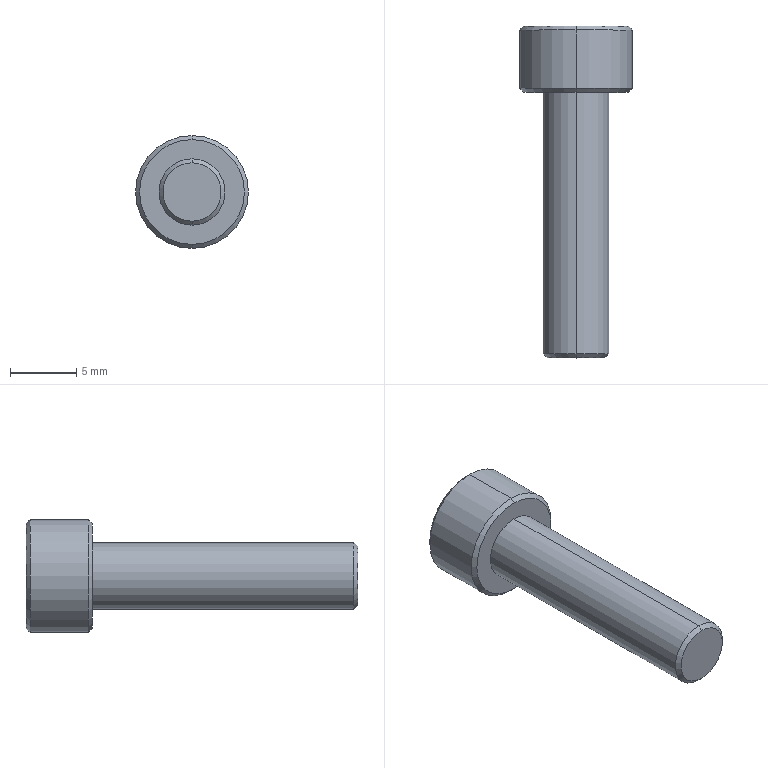Part | STEP file | Hex socket screw M5×20 | 1 solid | 28 faces | box 8.5 x 25 x 8.5 mm | volume 630.064 mm3 | plane 10 | cone 8 | spline 6 | cylinder 4 | commonest cylinder face diameters 5 x2 8.5 x2